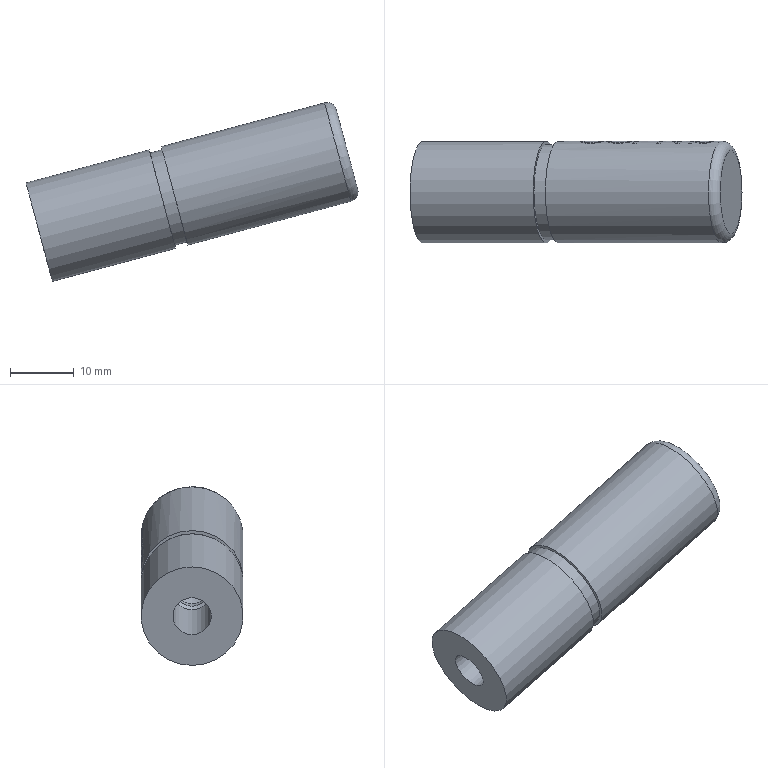Part | NX | features SGPN16-60_1 2 | 1 solid | 103 faces | box 52.1 x 16.001 x 28.059 mm | volume 9500 mm3 | plane 56 | cylinder 44 | cone 2 | torus 1 | commonest cylinder face diameters 15.8 x7 16 x4 1.309 x1 1.355 x1 1.621 x1 1.675 x1